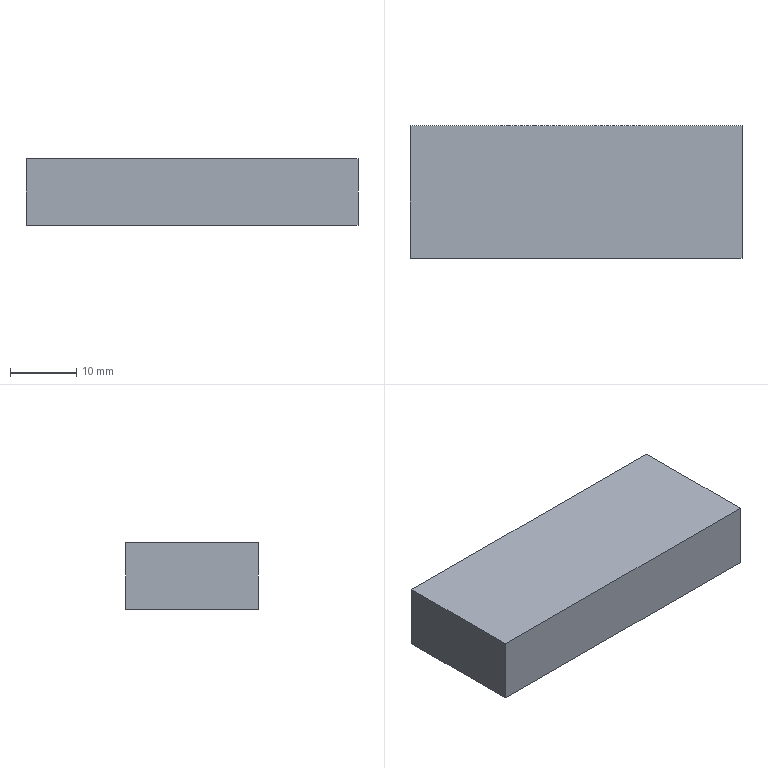Part | SolidWorks | features Extrusion 1 | 1 solid | 6 faces | box 50 x 20 x 10 mm | volume 10000 mm3 | plane 6
STEP:
#1=CARTESIAN_POINT('',(25.,-10.,0.));
#2=VERTEX_POINT('',#1);
#3=CARTESIAN_POINT('',(25.,10.,0.));
#4=VERTEX_POINT('',#3);
#5=CARTESIAN_POINT('',(25.,10.,0.));
#6=DIRECTION('',(0.,1.,0.));
#7=VECTOR('',#6,1000.);
#8=LINE('',#5,#7);
#9=EDGE_CURVE('',#2,#4,#8,.T.);
#10=ORIENTED_EDGE('',*,*,#9,.T.);
#11=CARTESIAN_POINT('',(25.,10.,10.));
#12=VERTEX_POINT('',#11);
#13=CARTESIAN_POINT('',(25.,10.,10.));
#14=DIRECTION('',(0.,0.,-1.));
#15=VECTOR('',#14,1000.);
#16=LINE('',#13,#15);
#17=EDGE_CURVE('',#12,#4,#16,.T.);
#18=ORIENTED_EDGE('',*,*,#17,.F.);
#19=CARTESIAN_POINT('',(25.,-10.,10.));
#20=VERTEX_POINT('',#19);
#21=CARTESIAN_POINT('',(25.,10.,10.));
#22=DIRECTION('',(0.,1.,0.));
#23=VECTOR('',#22,1000.);
#24=LINE('',#21,#23);
#25=EDGE_CURVE('',#20,#12,#24,.T.);
#26=ORIENTED_EDGE('',*,*,#25,.F.);
#27=CARTESIAN_POINT('',(25.,-10.,10.));
#28=DIRECTION('',(0.,0.,-1.));
#29=VECTOR('',#28,1000.);
#30=LINE('',#27,#29);
#31=EDGE_CURVE('',#20,#2,#30,.T.);
#32=ORIENTED_EDGE('',*,*,#31,.T.);
#33=EDGE_LOOP('',(#10,#18,#26,#32));
#34=FACE_OUTER_BOUND('',#33,.T.);
#35=CARTESIAN_POINT('',(25.,10.,10.));
#36=DIRECTION('',(-1.,0.,0.));
#37=DIRECTION('',(0.,-1.,0.));
#38=AXIS2_PLACEMENT_3D('',#35,#36,#37);
#39=PLANE('',#38);
#40=ADVANCED_FACE('',(#34),#39,.F.);
#41=CARTESIAN_POINT('',(-25.,10.,0.));
#42=VERTEX_POINT('',#41);
#43=CARTESIAN_POINT('',(-25.,10.,0.));
#44=DIRECTION('',(-1.,0.,0.));
#45=VECTOR('',#44,1000.);
#46=LINE('',#43,#45);
#47=EDGE_CURVE('',#4,#42,#46,.T.);
#48=ORIENTED_EDGE('',*,*,#47,.T.);
#49=CARTESIAN_POINT('',(-25.,10.,10.));
#50=VERTEX_POINT('',#49);
#51=CARTESIAN_POINT('',(-25.,10.,10.));
#52=DIRECTION('',(0.,0.,-1.));
#53=VECTOR('',#52,1000.);
#54=LINE('',#51,#53);
#55=EDGE_CURVE('',#50,#42,#54,.T.);
#56=ORIENTED_EDGE('',*,*,#55,.F.);
#57=CARTESIAN_POINT('',(-25.,10.,10.));
#58=DIRECTION('',(-1.,0.,0.));
#59=VECTOR('',#58,1000.);
#60=LINE('',#57,#59);
#61=EDGE_CURVE('',#12,#50,#60,.T.);
#62=ORIENTED_EDGE('',*,*,#61,.F.);
#63=ORIENTED_EDGE('',*,*,#17,.T.);
#64=EDGE_LOOP('',(#48,#56,#62,#63));
#65=FACE_OUTER_BOUND('',#64,.T.);
#66=CARTESIAN_POINT('',(-25.,10.,10.));
#67=DIRECTION('',(0.,-1.,0.));
#68=DIRECTION('',(0.,0.,-1.));
#69=AXIS2_PLACEMENT_3D('',#66,#67,#68);
#70=PLANE('',#69);
#71=ADVANCED_FACE('',(#65),#70,.F.);
#72=CARTESIAN_POINT('',(-25.,-10.,0.));
#73=VERTEX_POINT('',#72);
#74=CARTESIAN_POINT('',(-25.,10.,0.));
#75=DIRECTION('',(0.,-1.,0.));
#76=VECTOR('',#75,1000.);
#77=LINE('',#74,#76);
#78=EDGE_CURVE('',#42,#73,#77,.T.);
#79=ORIENTED_EDGE('',*,*,#78,.T.);
#80=CARTESIAN_POINT('',(-25.,-10.,10.));
#81=VERTEX_POINT('',#80);
#82=CARTESIAN_POINT('',(-25.,-10.,10.));
#83=DIRECTION('',(0.,0.,-1.));
#84=VECTOR('',#83,1000.);
#85=LINE('',#82,#84);
#86=EDGE_CURVE('',#81,#73,#85,.T.);
#87=ORIENTED_EDGE('',*,*,#86,.F.);
#88=CARTESIAN_POINT('',(-25.,10.,10.));
#89=DIRECTION('',(0.,-1.,0.));
#90=VECTOR('',#89,1000.);
#91=LINE('',#88,#90);
#92=EDGE_CURVE('',#50,#81,#91,.T.);
#93=ORIENTED_EDGE('',*,*,#92,.F.);
#94=ORIENTED_EDGE('',*,*,#55,.T.);
#95=EDGE_LOOP('',(#79,#87,#93,#94));
#96=FACE_OUTER_BOUND('',#95,.T.);
#97=CARTESIAN_POINT('',(-25.,10.,10.));
#98=DIRECTION('',(1.,0.,0.));
#99=DIRECTION('',(0.,1.,0.));
#100=AXIS2_PLACEMENT_3D('',#97,#98,#99);
#101=PLANE('',#100);
#102=ADVANCED_FACE('',(#96),#101,.F.);
#103=CARTESIAN_POINT('',(-25.,-10.,0.));
#104=DIRECTION('',(1.,0.,0.));
#105=VECTOR('',#104,1000.);
#106=LINE('',#103,#105);
#107=EDGE_CURVE('',#73,#2,#106,.T.);
#108=ORIENTED_EDGE('',*,*,#107,.T.);
#109=ORIENTED_EDGE('',*,*,#31,.F.);
#110=CARTESIAN_POINT('',(-25.,-10.,10.));
#111=DIRECTION('',(1.,0.,0.));
#112=VECTOR('',#111,1000.);
#113=LINE('',#110,#112);
#114=EDGE_CURVE('',#81,#20,#113,.T.);
#115=ORIENTED_EDGE('',*,*,#114,.F.);
#116=ORIENTED_EDGE('',*,*,#86,.T.);
#117=EDGE_LOOP('',(#108,#109,#115,#116));
#118=FACE_OUTER_BOUND('',#117,.T.);
#119=CARTESIAN_POINT('',(-25.,-10.,10.));
#120=DIRECTION('',(0.,1.,0.));
#121=DIRECTION('',(0.,0.,1.));
#122=AXIS2_PLACEMENT_3D('',#119,#120,#121);
#123=PLANE('',#122);
#124=ADVANCED_FACE('',(#118),#123,.F.);
#125=ORIENTED_EDGE('',*,*,#25,.T.);
#126=ORIENTED_EDGE('',*,*,#61,.T.);
#127=ORIENTED_EDGE('',*,*,#92,.T.);
#128=ORIENTED_EDGE('',*,*,#114,.T.);
#129=EDGE_LOOP('',(#125,#126,#127,#128));
#130=FACE_OUTER_BOUND('',#129,.T.);
#131=CARTESIAN_POINT('',(0.,0.,10.));
#132=DIRECTION('',(0.,0.,1.));
#133=DIRECTION('',(1.,0.,0.));
#134=AXIS2_PLACEMENT_3D('',#131,#132,#133);
#135=PLANE('',#134);
#136=ADVANCED_FACE('',(#130),#135,.T.);
#137=ORIENTED_EDGE('',*,*,#9,.F.);
#138=ORIENTED_EDGE('',*,*,#107,.F.);
#139=ORIENTED_EDGE('',*,*,#78,.F.);
#140=ORIENTED_EDGE('',*,*,#47,.F.);
#141=EDGE_LOOP('',(#137,#138,#139,#140));
#142=FACE_OUTER_BOUND('',#141,.T.);
#143=CARTESIAN_POINT('',(0.,0.,0.));
#144=DIRECTION('',(0.,0.,1.));
#145=DIRECTION('',(1.,0.,0.));
#146=AXIS2_PLACEMENT_3D('',#143,#144,#145);
#147=PLANE('',#146);
#148=ADVANCED_FACE('',(#142),#147,.F.);
#149=CLOSED_SHELL('',(#40,#71,#102,#124,#136,#148));
#150=MANIFOLD_SOLID_BREP('',#149);
#151=CARTESIAN_POINT('',(0.,0.,0.));
#152=DIRECTION('',(0.,0.,1.));
#153=DIRECTION('',(1.,0.,0.));
#154=AXIS2_PLACEMENT_3D('',#151,#152,#153);
#155=(LENGTH_UNIT()NAMED_UNIT(*)SI_UNIT(.MILLI.,.METRE.));
#156=UNCERTAINTY_MEASURE_WITH_UNIT(LENGTH_MEASURE(0.00001),#155,'','');
#157=(NAMED_UNIT(*)PLANE_ANGLE_UNIT()SI_UNIT($,.RADIAN.));
#158=(NAMED_UNIT(*)SI_UNIT($,.STERADIAN.)SOLID_ANGLE_UNIT());
#159=(GEOMETRIC_REPRESENTATION_CONTEXT(3)GLOBAL_UNCERTAINTY_ASSIGNED_CONTEXT((#156))GLOBAL_UNIT_ASSIGNED_CONTEXT((#155,#157,#158))REPRESENTATION_CONTEXT('',''));
#160=ADVANCED_BREP_SHAPE_REPRESENTATION('',(#150,#154),#159);